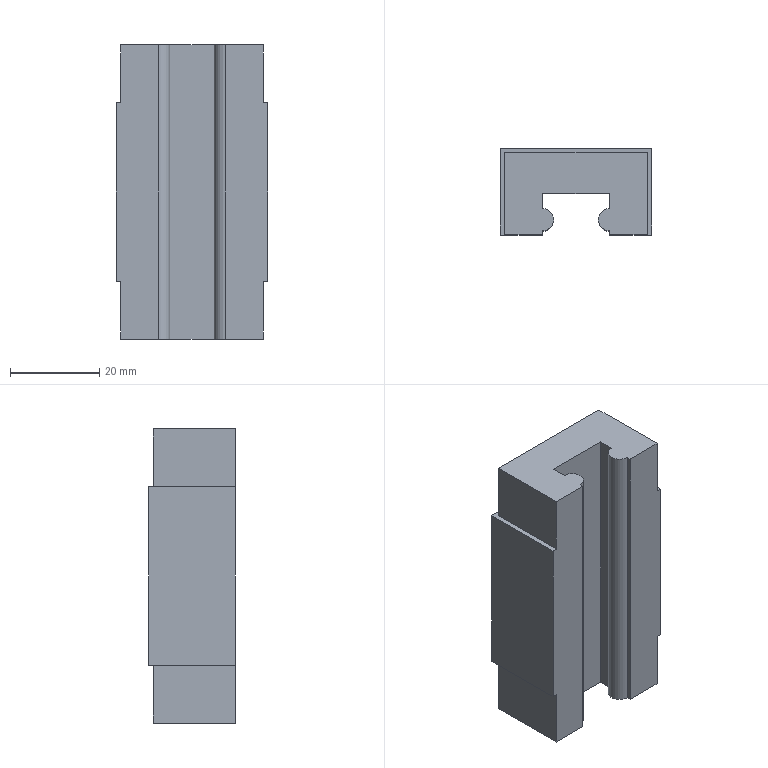Part | Creo | features CURVE 3, DATUM PLANE 3, PROTRUSION 2, COORDINATE SYSTEM 1, CUT 1 | 1 solid | 34 faces | box 34 x 19.41 x 66 mm | volume 33431 mm3 | plane 24 | cylinder 10 | commonest cylinder face diameters 3.3 x8 5 x2
STEP:
#1=CARTESIAN_POINT('',(0.,0.,0.));
#2=DIRECTION('',(0.,0.,1.));
#3=DIRECTION('',(1.,0.,0.));
#4=AXIS2_PLACEMENT_3D('',#1,#2,#3);
#5=CARTESIAN_POINT('',(16.,0.,-20.));
#6=VERTEX_POINT('',#5);
#7=CARTESIAN_POINT('',(16.,18.41,-20.));
#8=VERTEX_POINT('',#7);
#9=CARTESIAN_POINT('',(16.,0.,-20.));
#10=DIRECTION('',(0.,1.,0.));
#11=VECTOR('',#10,18.41);
#12=LINE('',#9,#11);
#13=EDGE_CURVE('',#6,#8,#12,.T.);
#14=ORIENTED_EDGE('',*,*,#13,.F.);
#15=CARTESIAN_POINT('',(17.,0.,-20.));
#16=VERTEX_POINT('',#15);
#17=CARTESIAN_POINT('',(16.,0.,-20.));
#18=DIRECTION('',(1.,0.,0.));
#19=VECTOR('',#18,1.);
#20=LINE('',#17,#19);
#21=EDGE_CURVE('',#6,#16,#20,.T.);
#22=ORIENTED_EDGE('',*,*,#21,.T.);
#23=CARTESIAN_POINT('',(17.,19.41,-20.));
#24=VERTEX_POINT('',#23);
#25=CARTESIAN_POINT('',(17.,0.,-20.));
#26=DIRECTION('',(0.,1.,0.));
#27=VECTOR('',#26,19.41);
#28=LINE('',#25,#27);
#29=EDGE_CURVE('',#16,#24,#28,.T.);
#30=ORIENTED_EDGE('',*,*,#29,.T.);
#31=CARTESIAN_POINT('',(-17.,19.41,-20.));
#32=VERTEX_POINT('',#31);
#33=CARTESIAN_POINT('',(17.,19.41,-20.));
#34=DIRECTION('',(-1.,0.,0.));
#35=VECTOR('',#34,34.);
#36=LINE('',#33,#35);
#37=EDGE_CURVE('',#24,#32,#36,.T.);
#38=ORIENTED_EDGE('',*,*,#37,.T.);
#39=CARTESIAN_POINT('',(-17.,0.,-20.));
#40=VERTEX_POINT('',#39);
#41=CARTESIAN_POINT('',(-17.,19.41,-20.));
#42=DIRECTION('',(0.,-1.,0.));
#43=VECTOR('',#42,19.41);
#44=LINE('',#41,#43);
#45=EDGE_CURVE('',#32,#40,#44,.T.);
#46=ORIENTED_EDGE('',*,*,#45,.T.);
#47=CARTESIAN_POINT('',(-16.,0.,-20.));
#48=VERTEX_POINT('',#47);
#49=CARTESIAN_POINT('',(-17.,0.,-20.));
#50=DIRECTION('',(1.,0.,0.));
#51=VECTOR('',#50,1.);
#52=LINE('',#49,#51);
#53=EDGE_CURVE('',#40,#48,#52,.T.);
#54=ORIENTED_EDGE('',*,*,#53,.T.);
#55=CARTESIAN_POINT('',(-16.,18.41,-20.));
#56=VERTEX_POINT('',#55);
#57=CARTESIAN_POINT('',(-16.,0.,-20.));
#58=DIRECTION('',(0.,1.,0.));
#59=VECTOR('',#58,18.41);
#60=LINE('',#57,#59);
#61=EDGE_CURVE('',#48,#56,#60,.T.);
#62=ORIENTED_EDGE('',*,*,#61,.T.);
#63=CARTESIAN_POINT('',(16.,18.41,-20.));
#64=DIRECTION('',(-1.,0.,0.));
#65=VECTOR('',#64,32.);
#66=LINE('',#63,#65);
#67=EDGE_CURVE('',#8,#56,#66,.T.);
#68=ORIENTED_EDGE('',*,*,#67,.F.);
#69=EDGE_LOOP('',(#14,#22,#30,#38,#46,#54,#62,#68));
#70=FACE_OUTER_BOUND('',#69,.F.);
#71=CARTESIAN_POINT('',(0.,0.,-20.));
#72=DIRECTION('',(0.,0.,1.));
#73=DIRECTION('',(1.,0.,0.));
#74=AXIS2_PLACEMENT_3D('',#71,#72,#73);
#75=PLANE('',#74);
#76=ADVANCED_FACE('',(#70),#75,.F.);
#77=ORIENTED_EDGE('',*,*,#13,.T.);
#78=CARTESIAN_POINT('',(16.,18.41,-33.));
#79=VERTEX_POINT('',#78);
#80=CARTESIAN_POINT('',(16.,18.41,-33.));
#81=DIRECTION('',(0.,0.,1.));
#82=VECTOR('',#81,13.);
#83=LINE('',#80,#82);
#84=EDGE_CURVE('',#79,#8,#83,.T.);
#85=ORIENTED_EDGE('',*,*,#84,.F.);
#86=CARTESIAN_POINT('',(16.,0.,-33.));
#87=VERTEX_POINT('',#86);
#88=CARTESIAN_POINT('',(16.,0.,-33.));
#89=DIRECTION('',(0.,1.,0.));
#90=VECTOR('',#89,18.41);
#91=LINE('',#88,#90);
#92=EDGE_CURVE('',#87,#79,#91,.T.);
#93=ORIENTED_EDGE('',*,*,#92,.F.);
#94=CARTESIAN_POINT('',(16.,0.,-33.));
#95=DIRECTION('',(0.,0.,1.));
#96=VECTOR('',#95,13.);
#97=LINE('',#94,#96);
#98=EDGE_CURVE('',#87,#6,#97,.T.);
#99=ORIENTED_EDGE('',*,*,#98,.T.);
#100=EDGE_LOOP('',(#77,#85,#93,#99));
#101=FACE_OUTER_BOUND('',#100,.F.);
#102=CARTESIAN_POINT('',(16.,0.,-33.));
#103=DIRECTION('',(1.,0.,0.));
#104=DIRECTION('',(0.,1.,0.));
#105=AXIS2_PLACEMENT_3D('',#102,#103,#104);
#106=PLANE('',#105);
#107=ADVANCED_FACE('',(#101),#106,.T.);
#108=CARTESIAN_POINT('',(16.,0.,20.));
#109=VERTEX_POINT('',#108);
#110=CARTESIAN_POINT('',(16.,18.41,20.));
#111=VERTEX_POINT('',#110);
#112=CARTESIAN_POINT('',(16.,0.,20.));
#113=DIRECTION('',(0.,1.,0.));
#114=VECTOR('',#113,18.41);
#115=LINE('',#112,#114);
#116=EDGE_CURVE('',#109,#111,#115,.T.);
#117=ORIENTED_EDGE('',*,*,#116,.F.);
#118=CARTESIAN_POINT('',(16.,0.,33.));
#119=VERTEX_POINT('',#118);
#120=CARTESIAN_POINT('',(16.,0.,20.));
#121=DIRECTION('',(0.,0.,1.));
#122=VECTOR('',#121,13.);
#123=LINE('',#120,#122);
#124=EDGE_CURVE('',#109,#119,#123,.T.);
#125=ORIENTED_EDGE('',*,*,#124,.T.);
#126=CARTESIAN_POINT('',(16.,18.41,33.));
#127=VERTEX_POINT('',#126);
#128=CARTESIAN_POINT('',(16.,0.,33.));
#129=DIRECTION('',(0.,1.,0.));
#130=VECTOR('',#129,18.41);
#131=LINE('',#128,#130);
#132=EDGE_CURVE('',#119,#127,#131,.T.);
#133=ORIENTED_EDGE('',*,*,#132,.T.);
#134=CARTESIAN_POINT('',(16.,18.41,20.));
#135=DIRECTION('',(0.,0.,1.));
#136=VECTOR('',#135,13.);
#137=LINE('',#134,#136);
#138=EDGE_CURVE('',#111,#127,#137,.T.);
#139=ORIENTED_EDGE('',*,*,#138,.F.);
#140=EDGE_LOOP('',(#117,#125,#133,#139));
#141=FACE_OUTER_BOUND('',#140,.F.);
#142=CARTESIAN_POINT('',(16.,0.,-33.));
#143=DIRECTION('',(1.,0.,0.));
#144=DIRECTION('',(0.,1.,0.));
#145=AXIS2_PLACEMENT_3D('',#142,#143,#144);
#146=PLANE('',#145);
#147=ADVANCED_FACE('',(#141),#146,.T.);
#148=ORIENTED_EDGE('',*,*,#67,.T.);
#149=CARTESIAN_POINT('',(-16.,18.41,-33.));
#150=VERTEX_POINT('',#149);
#151=CARTESIAN_POINT('',(-16.,18.41,-33.));
#152=DIRECTION('',(0.,0.,1.));
#153=VECTOR('',#152,13.);
#154=LINE('',#151,#153);
#155=EDGE_CURVE('',#150,#56,#154,.T.);
#156=ORIENTED_EDGE('',*,*,#155,.F.);
#157=CARTESIAN_POINT('',(16.,18.41,-33.));
#158=DIRECTION('',(-1.,0.,0.));
#159=VECTOR('',#158,32.);
#160=LINE('',#157,#159);
#161=EDGE_CURVE('',#79,#150,#160,.T.);
#162=ORIENTED_EDGE('',*,*,#161,.F.);
#163=ORIENTED_EDGE('',*,*,#84,.T.);
#164=EDGE_LOOP('',(#148,#156,#162,#163));
#165=FACE_OUTER_BOUND('',#164,.F.);
#166=CARTESIAN_POINT('',(16.,18.41,-33.));
#167=DIRECTION('',(0.,1.,0.));
#168=DIRECTION('',(-1.,0.,0.));
#169=AXIS2_PLACEMENT_3D('',#166,#167,#168);
#170=PLANE('',#169);
#171=ADVANCED_FACE('',(#165),#170,.T.);
#172=CARTESIAN_POINT('',(-16.,18.41,20.));
#173=VERTEX_POINT('',#172);
#174=CARTESIAN_POINT('',(16.,18.41,20.));
#175=DIRECTION('',(-1.,0.,0.));
#176=VECTOR('',#175,32.);
#177=LINE('',#174,#176);
#178=EDGE_CURVE('',#111,#173,#177,.T.);
#179=ORIENTED_EDGE('',*,*,#178,.F.);
#180=ORIENTED_EDGE('',*,*,#138,.T.);
#181=CARTESIAN_POINT('',(-16.,18.41,33.));
#182=VERTEX_POINT('',#181);
#183=CARTESIAN_POINT('',(16.,18.41,33.));
#184=DIRECTION('',(-1.,0.,0.));
#185=VECTOR('',#184,32.);
#186=LINE('',#183,#185);
#187=EDGE_CURVE('',#127,#182,#186,.T.);
#188=ORIENTED_EDGE('',*,*,#187,.T.);
#189=CARTESIAN_POINT('',(-16.,18.41,20.));
#190=DIRECTION('',(0.,0.,1.));
#191=VECTOR('',#190,13.);
#192=LINE('',#189,#191);
#193=EDGE_CURVE('',#173,#182,#192,.T.);
#194=ORIENTED_EDGE('',*,*,#193,.F.);
#195=EDGE_LOOP('',(#179,#180,#188,#194));
#196=FACE_OUTER_BOUND('',#195,.F.);
#197=CARTESIAN_POINT('',(16.,18.41,-33.));
#198=DIRECTION('',(0.,1.,0.));
#199=DIRECTION('',(-1.,0.,0.));
#200=AXIS2_PLACEMENT_3D('',#197,#198,#199);
#201=PLANE('',#200);
#202=ADVANCED_FACE('',(#196),#201,.T.);
#203=ORIENTED_EDGE('',*,*,#61,.F.);
#204=CARTESIAN_POINT('',(-16.,0.,-33.));
#205=VERTEX_POINT('',#204);
#206=CARTESIAN_POINT('',(-16.,0.,-33.));
#207=DIRECTION('',(0.,0.,1.));
#208=VECTOR('',#207,13.);
#209=LINE('',#206,#208);
#210=EDGE_CURVE('',#205,#48,#209,.T.);
#211=ORIENTED_EDGE('',*,*,#210,.F.);
#212=CARTESIAN_POINT('',(-16.,18.41,-33.));
#213=DIRECTION('',(0.,-1.,0.));
#214=VECTOR('',#213,18.41);
#215=LINE('',#212,#214);
#216=EDGE_CURVE('',#150,#205,#215,.T.);
#217=ORIENTED_EDGE('',*,*,#216,.F.);
#218=ORIENTED_EDGE('',*,*,#155,.T.);
#219=EDGE_LOOP('',(#203,#211,#217,#218));
#220=FACE_OUTER_BOUND('',#219,.F.);
#221=CARTESIAN_POINT('',(-16.,18.41,-33.));
#222=DIRECTION('',(-1.,0.,0.));
#223=DIRECTION('',(0.,-1.,0.));
#224=AXIS2_PLACEMENT_3D('',#221,#222,#223);
#225=PLANE('',#224);
#226=ADVANCED_FACE('',(#220),#225,.T.);
#227=CARTESIAN_POINT('',(-16.,0.,20.));
#228=VERTEX_POINT('',#227);
#229=CARTESIAN_POINT('',(-16.,0.,20.));
#230=DIRECTION('',(0.,1.,0.));
#231=VECTOR('',#230,18.41);
#232=LINE('',#229,#231);
#233=EDGE_CURVE('',#228,#173,#232,.T.);
#234=ORIENTED_EDGE('',*,*,#233,.T.);
#235=ORIENTED_EDGE('',*,*,#193,.T.);
#236=CARTESIAN_POINT('',(-16.,0.,33.));
#237=VERTEX_POINT('',#236);
#238=CARTESIAN_POINT('',(-16.,18.41,33.));
#239=DIRECTION('',(0.,-1.,0.));
#240=VECTOR('',#239,18.41);
#241=LINE('',#238,#240);
#242=EDGE_CURVE('',#182,#237,#241,.T.);
#243=ORIENTED_EDGE('',*,*,#242,.T.);
#244=CARTESIAN_POINT('',(-16.,0.,20.));
#245=DIRECTION('',(0.,0.,1.));
#246=VECTOR('',#245,13.);
#247=LINE('',#244,#246);
#248=EDGE_CURVE('',#228,#237,#247,.T.);
#249=ORIENTED_EDGE('',*,*,#248,.F.);
#250=EDGE_LOOP('',(#234,#235,#243,#249));
#251=FACE_OUTER_BOUND('',#250,.F.);
#252=CARTESIAN_POINT('',(-16.,18.41,-33.));
#253=DIRECTION('',(-1.,0.,0.));
#254=DIRECTION('',(0.,-1.,0.));
#255=AXIS2_PLACEMENT_3D('',#252,#253,#254);
#256=PLANE('',#255);
#257=ADVANCED_FACE('',(#251),#256,.T.);
#258=CARTESIAN_POINT('',(-17.,0.,20.));
#259=VERTEX_POINT('',#258);
#260=CARTESIAN_POINT('',(-17.,0.,20.));
#261=DIRECTION('',(1.,0.,0.));
#262=VECTOR('',#261,1.);
#263=LINE('',#260,#262);
#264=EDGE_CURVE('',#259,#228,#263,.T.);
#265=ORIENTED_EDGE('',*,*,#264,.T.);
#266=ORIENTED_EDGE('',*,*,#248,.T.);
#267=CARTESIAN_POINT('',(-7.5,0.,33.));
#268=VERTEX_POINT('',#267);
#269=CARTESIAN_POINT('',(-16.,0.,33.));
#270=DIRECTION('',(1.,0.,0.));
#271=VECTOR('',#270,8.5);
#272=LINE('',#269,#271);
#273=EDGE_CURVE('',#237,#268,#272,.T.);
#274=ORIENTED_EDGE('',*,*,#273,.T.);
#275=CARTESIAN_POINT('',(-7.5,0.,-33.));
#276=VERTEX_POINT('',#275);
#277=CARTESIAN_POINT('',(-7.5,0.,-33.));
#278=DIRECTION('',(0.,0.,1.));
#279=VECTOR('',#278,66.);
#280=LINE('',#277,#279);
#281=EDGE_CURVE('',#276,#268,#280,.T.);
#282=ORIENTED_EDGE('',*,*,#281,.F.);
#283=CARTESIAN_POINT('',(-16.,0.,-33.));
#284=DIRECTION('',(1.,0.,0.));
#285=VECTOR('',#284,8.5);
#286=LINE('',#283,#285);
#287=EDGE_CURVE('',#205,#276,#286,.T.);
#288=ORIENTED_EDGE('',*,*,#287,.F.);
#289=ORIENTED_EDGE('',*,*,#210,.T.);
#290=ORIENTED_EDGE('',*,*,#53,.F.);
#291=CARTESIAN_POINT('',(-17.,0.,-20.));
#292=DIRECTION('',(0.,0.,1.));
#293=VECTOR('',#292,40.);
#294=LINE('',#291,#293);
#295=EDGE_CURVE('',#40,#259,#294,.T.);
#296=ORIENTED_EDGE('',*,*,#295,.T.);
#297=EDGE_LOOP('',(#265,#266,#274,#282,#288,#289,#290,#296));
#298=FACE_OUTER_BOUND('',#297,.F.);
#299=CARTESIAN_POINT('',(-17.,0.,-20.));
#300=DIRECTION('',(0.,-1.,0.));
#301=DIRECTION('',(1.,0.,0.));
#302=AXIS2_PLACEMENT_3D('',#299,#300,#301);
#303=PLANE('',#302);
#304=ADVANCED_FACE('',(#298),#303,.T.);
#305=ORIENTED_EDGE('',*,*,#116,.T.);
#306=ORIENTED_EDGE('',*,*,#178,.T.);
#307=ORIENTED_EDGE('',*,*,#233,.F.);
#308=ORIENTED_EDGE('',*,*,#264,.F.);
#309=CARTESIAN_POINT('',(-17.,19.41,20.));
#310=VERTEX_POINT('',#309);
#311=CARTESIAN_POINT('',(-17.,19.41,20.));
#312=DIRECTION('',(0.,-1.,0.));
#313=VECTOR('',#312,19.41);
#314=LINE('',#311,#313);
#315=EDGE_CURVE('',#310,#259,#314,.T.);
#316=ORIENTED_EDGE('',*,*,#315,.F.);
#317=CARTESIAN_POINT('',(17.,19.41,20.));
#318=VERTEX_POINT('',#317);
#319=CARTESIAN_POINT('',(17.,19.41,20.));
#320=DIRECTION('',(-1.,0.,0.));
#321=VECTOR('',#320,34.);
#322=LINE('',#319,#321);
#323=EDGE_CURVE('',#318,#310,#322,.T.);
#324=ORIENTED_EDGE('',*,*,#323,.F.);
#325=CARTESIAN_POINT('',(17.,0.,20.));
#326=VERTEX_POINT('',#325);
#327=CARTESIAN_POINT('',(17.,0.,20.));
#328=DIRECTION('',(0.,1.,0.));
#329=VECTOR('',#328,19.41);
#330=LINE('',#327,#329);
#331=EDGE_CURVE('',#326,#318,#330,.T.);
#332=ORIENTED_EDGE('',*,*,#331,.F.);
#333=CARTESIAN_POINT('',(16.,0.,20.));
#334=DIRECTION('',(1.,0.,0.));
#335=VECTOR('',#334,1.);
#336=LINE('',#333,#335);
#337=EDGE_CURVE('',#109,#326,#336,.T.);
#338=ORIENTED_EDGE('',*,*,#337,.F.);
#339=EDGE_LOOP('',(#305,#306,#307,#308,#316,#324,#332,#338));
#340=FACE_OUTER_BOUND('',#339,.F.);
#341=CARTESIAN_POINT('',(0.,0.,20.));
#342=DIRECTION('',(0.,0.,1.));
#343=DIRECTION('',(1.,0.,0.));
#344=AXIS2_PLACEMENT_3D('',#341,#342,#343);
#345=PLANE('',#344);
#346=ADVANCED_FACE('',(#340),#345,.T.);
#347=ORIENTED_EDGE('',*,*,#45,.F.);
#348=CARTESIAN_POINT('',(-17.,19.41,-20.));
#349=DIRECTION('',(0.,0.,1.));
#350=VECTOR('',#349,40.);
#351=LINE('',#348,#350);
#352=EDGE_CURVE('',#32,#310,#351,.T.);
#353=ORIENTED_EDGE('',*,*,#352,.T.);
#354=ORIENTED_EDGE('',*,*,#315,.T.);
#355=ORIENTED_EDGE('',*,*,#295,.F.);
#356=EDGE_LOOP('',(#347,#353,#354,#355));
#357=FACE_OUTER_BOUND('',#356,.F.);
#358=CARTESIAN_POINT('',(-17.,19.41,-20.));
#359=DIRECTION('',(-1.,0.,0.));
#360=DIRECTION('',(0.,-1.,0.));
#361=AXIS2_PLACEMENT_3D('',#358,#359,#360);
#362=PLANE('',#361);
#363=ADVANCED_FACE('',(#357),#362,.T.);
#364=ORIENTED_EDGE('',*,*,#37,.F.);
#365=CARTESIAN_POINT('',(17.,19.41,-20.));
#366=DIRECTION('',(0.,0.,1.));
#367=VECTOR('',#366,40.);
#368=LINE('',#365,#367);
#369=EDGE_CURVE('',#24,#318,#368,.T.);
#370=ORIENTED_EDGE('',*,*,#369,.T.);
#371=ORIENTED_EDGE('',*,*,#323,.T.);
#372=ORIENTED_EDGE('',*,*,#352,.F.);
#373=EDGE_LOOP('',(#364,#370,#371,#372));
#374=FACE_OUTER_BOUND('',#373,.F.);
#375=CARTESIAN_POINT('',(14.65,19.41,-13.));
#376=VERTEX_POINT('',#375);
#377=CARTESIAN_POINT('',(11.35,19.41,-13.));
#378=VERTEX_POINT('',#377);
#379=CARTESIAN_POINT('',(13.,19.41,-13.));
#380=DIRECTION('',(0.,1.,0.));
#381=DIRECTION('',(1.,0.,0.));
#382=AXIS2_PLACEMENT_3D('',#379,#380,#381);
#383=CIRCLE('',#382,1.65);
#384=EDGE_CURVE('',#376,#378,#383,.T.);
#385=ORIENTED_EDGE('',*,*,#384,.T.);
#386=CARTESIAN_POINT('',(13.,19.41,-13.));
#387=DIRECTION('',(0.,1.,0.));
#388=DIRECTION('',(-1.,0.,0.));
#389=AXIS2_PLACEMENT_3D('',#386,#387,#388);
#390=CIRCLE('',#389,1.65);
#391=EDGE_CURVE('',#378,#376,#390,.T.);
#392=ORIENTED_EDGE('',*,*,#391,.T.);
#393=EDGE_LOOP('',(#385,#392));
#394=FACE_BOUND('',#393,.F.);
#395=CARTESIAN_POINT('',(-11.35,19.41,-13.));
#396=VERTEX_POINT('',#395);
#397=CARTESIAN_POINT('',(-14.65,19.41,-13.));
#398=VERTEX_POINT('',#397);
#399=CARTESIAN_POINT('',(-13.,19.41,-13.));
#400=DIRECTION('',(0.,1.,0.));
#401=DIRECTION('',(1.,0.,0.));
#402=AXIS2_PLACEMENT_3D('',#399,#400,#401);
#403=CIRCLE('',#402,1.65);
#404=EDGE_CURVE('',#396,#398,#403,.T.);
#405=ORIENTED_EDGE('',*,*,#404,.T.);
#406=CARTESIAN_POINT('',(-13.,19.41,-13.));
#407=DIRECTION('',(0.,1.,0.));
#408=DIRECTION('',(-1.,0.,0.));
#409=AXIS2_PLACEMENT_3D('',#406,#407,#408);
#410=CIRCLE('',#409,1.65);
#411=EDGE_CURVE('',#398,#396,#410,.T.);
#412=ORIENTED_EDGE('',*,*,#411,.T.);
#413=EDGE_LOOP('',(#405,#412));
#414=FACE_BOUND('',#413,.F.);
#415=CARTESIAN_POINT('',(-11.35,19.41,13.));
#416=VERTEX_POINT('',#415);
#417=CARTESIAN_POINT('',(-14.65,19.41,13.));
#418=VERTEX_POINT('',#417);
#419=CARTESIAN_POINT('',(-13.,19.41,13.));
#420=DIRECTION('',(0.,1.,0.));
#421=DIRECTION('',(1.,0.,0.));
#422=AXIS2_PLACEMENT_3D('',#419,#420,#421);
#423=CIRCLE('',#422,1.65);
#424=EDGE_CURVE('',#416,#418,#423,.T.);
#425=ORIENTED_EDGE('',*,*,#424,.T.);
#426=CARTESIAN_POINT('',(-13.,19.41,13.));
#427=DIRECTION('',(0.,1.,0.));
#428=DIRECTION('',(-1.,0.,0.));
#429=AXIS2_PLACEMENT_3D('',#426,#427,#428);
#430=CIRCLE('',#429,1.65);
#431=EDGE_CURVE('',#418,#416,#430,.T.);
#432=ORIENTED_EDGE('',*,*,#431,.T.);
#433=EDGE_LOOP('',(#425,#432));
#434=FACE_BOUND('',#433,.F.);
#435=CARTESIAN_POINT('',(14.65,19.41,13.));
#436=VERTEX_POINT('',#435);
#437=CARTESIAN_POINT('',(11.35,19.41,13.));
#438=VERTEX_POINT('',#437);
#439=CARTESIAN_POINT('',(13.,19.41,13.));
#440=DIRECTION('',(0.,1.,0.));
#441=DIRECTION('',(1.,0.,0.));
#442=AXIS2_PLACEMENT_3D('',#439,#440,#441);
#443=CIRCLE('',#442,1.65);
#444=EDGE_CURVE('',#436,#438,#443,.T.);
#445=ORIENTED_EDGE('',*,*,#444,.T.);
#446=CARTESIAN_POINT('',(13.,19.41,13.));
#447=DIRECTION('',(0.,1.,0.));
#448=DIRECTION('',(-1.,0.,0.));
#449=AXIS2_PLACEMENT_3D('',#446,#447,#448);
#450=CIRCLE('',#449,1.65);
#451=EDGE_CURVE('',#438,#436,#450,.T.);
#452=ORIENTED_EDGE('',*,*,#451,.T.);
#453=EDGE_LOOP('',(#445,#452));
#454=FACE_BOUND('',#453,.F.);
#455=CARTESIAN_POINT('',(17.,19.41,-20.));
#456=DIRECTION('',(0.,1.,0.));
#457=DIRECTION('',(-1.,0.,0.));
#458=AXIS2_PLACEMENT_3D('',#455,#456,#457);
#459=PLANE('',#458);
#460=ADVANCED_FACE('',(#374,#394,#414,#434,#454),#459,.T.);
#461=ORIENTED_EDGE('',*,*,#29,.F.);
#462=CARTESIAN_POINT('',(17.,0.,-20.));
#463=DIRECTION('',(0.,0.,1.));
#464=VECTOR('',#463,40.);
#465=LINE('',#462,#464);
#466=EDGE_CURVE('',#16,#326,#465,.T.);
#467=ORIENTED_EDGE('',*,*,#466,.T.);
#468=ORIENTED_EDGE('',*,*,#331,.T.);
#469=ORIENTED_EDGE('',*,*,#369,.F.);
#470=EDGE_LOOP('',(#461,#467,#468,#469));
#471=FACE_OUTER_BOUND('',#470,.F.);
#472=CARTESIAN_POINT('',(17.,0.,-20.));
#473=DIRECTION('',(1.,0.,0.));
#474=DIRECTION('',(0.,1.,0.));
#475=AXIS2_PLACEMENT_3D('',#472,#473,#474);
#476=PLANE('',#475);
#477=ADVANCED_FACE('',(#471),#476,.T.);
#478=CARTESIAN_POINT('',(7.5,0.,-33.));
#479=VERTEX_POINT('',#478);
#480=CARTESIAN_POINT('',(7.5,0.,33.));
#481=VERTEX_POINT('',#480);
#482=CARTESIAN_POINT('',(7.5,0.,-33.));
#483=DIRECTION('',(0.,0.,1.));
#484=VECTOR('',#483,66.);
#485=LINE('',#482,#484);
#486=EDGE_CURVE('',#479,#481,#485,.T.);
#487=ORIENTED_EDGE('',*,*,#486,.T.);
#488=CARTESIAN_POINT('',(7.5,0.,33.));
#489=DIRECTION('',(1.,0.,0.));
#490=VECTOR('',#489,8.5);
#491=LINE('',#488,#490);
#492=EDGE_CURVE('',#481,#119,#491,.T.);
#493=ORIENTED_EDGE('',*,*,#492,.T.);
#494=ORIENTED_EDGE('',*,*,#124,.F.);
#495=ORIENTED_EDGE('',*,*,#337,.T.);
#496=ORIENTED_EDGE('',*,*,#466,.F.);
#497=ORIENTED_EDGE('',*,*,#21,.F.);
#498=ORIENTED_EDGE('',*,*,#98,.F.);
#499=CARTESIAN_POINT('',(7.5,0.,-33.));
#500=DIRECTION('',(1.,0.,0.));
#501=VECTOR('',#500,8.5);
#502=LINE('',#499,#501);
#503=EDGE_CURVE('',#479,#87,#502,.T.);
#504=ORIENTED_EDGE('',*,*,#503,.F.);
#505=EDGE_LOOP('',(#487,#493,#494,#495,#496,#497,#498,#504));
#506=FACE_OUTER_BOUND('',#505,.F.);
#507=CARTESIAN_POINT('',(7.5,0.,-20.));
#508=DIRECTION('',(0.,-1.,0.));
#509=DIRECTION('',(1.,0.,0.));
#510=AXIS2_PLACEMENT_3D('',#507,#508,#509);
#511=PLANE('',#510);
#512=ADVANCED_FACE('',(#506),#511,.T.);
#513=CARTESIAN_POINT('',(7.5,0.9,-33.));
#514=VERTEX_POINT('',#513);
#515=CARTESIAN_POINT('',(7.5,0.9,33.));
#516=VERTEX_POINT('',#515);
#517=CARTESIAN_POINT('',(7.5,0.9,-33.));
#518=DIRECTION('',(0.,0.,1.));
#519=VECTOR('',#518,66.);
#520=LINE('',#517,#519);
#521=EDGE_CURVE('',#514,#516,#520,.T.);
#522=ORIENTED_EDGE('',*,*,#521,.T.);
#523=CARTESIAN_POINT('',(7.5,0.9,33.));
#524=DIRECTION('',(0.,-1.,0.));
#525=VECTOR('',#524,0.9);
#526=LINE('',#523,#525);
#527=EDGE_CURVE('',#516,#481,#526,.T.);
#528=ORIENTED_EDGE('',*,*,#527,.T.);
#529=ORIENTED_EDGE('',*,*,#486,.F.);
#530=CARTESIAN_POINT('',(7.5,0.9,-33.));
#531=DIRECTION('',(0.,-1.,0.));
#532=VECTOR('',#531,0.9);
#533=LINE('',#530,#532);
#534=EDGE_CURVE('',#514,#479,#533,.T.);
#535=ORIENTED_EDGE('',*,*,#534,.F.);
#536=EDGE_LOOP('',(#522,#528,#529,#535));
#537=FACE_OUTER_BOUND('',#536,.F.);
#538=CARTESIAN_POINT('',(7.5,0.9,-20.));
#539=DIRECTION('',(-1.,0.,0.));
#540=DIRECTION('',(0.,-1.,0.));
#541=AXIS2_PLACEMENT_3D('',#538,#539,#540);
#542=PLANE('',#541);
#543=ADVANCED_FACE('',(#537),#542,.T.);
#544=CARTESIAN_POINT('',(7.5,5.9,-33.));
#545=VERTEX_POINT('',#544);
#546=CARTESIAN_POINT('',(7.5,5.9,33.));
#547=VERTEX_POINT('',#546);
#548=CARTESIAN_POINT('',(7.5,5.9,-33.));
#549=DIRECTION('',(0.,0.,1.));
#550=VECTOR('',#549,66.);
#551=LINE('',#548,#550);
#552=EDGE_CURVE('',#545,#547,#551,.T.);
#553=ORIENTED_EDGE('',*,*,#552,.T.);
#554=CARTESIAN_POINT('',(7.5,3.4,33.));
#555=DIRECTION('',(0.,0.,1.));
#556=DIRECTION('',(0.,1.,0.));
#557=AXIS2_PLACEMENT_3D('',#554,#555,#556);
#558=CIRCLE('',#557,2.5);
#559=EDGE_CURVE('',#547,#516,#558,.T.);
#560=ORIENTED_EDGE('',*,*,#559,.T.);
#561=ORIENTED_EDGE('',*,*,#521,.F.);
#562=CARTESIAN_POINT('',(7.5,3.4,-33.));
#563=DIRECTION('',(0.,0.,1.));
#564=DIRECTION('',(0.,1.,0.));
#565=AXIS2_PLACEMENT_3D('',#562,#563,#564);
#566=CIRCLE('',#565,2.5);
#567=EDGE_CURVE('',#545,#514,#566,.T.);
#568=ORIENTED_EDGE('',*,*,#567,.F.);
#569=EDGE_LOOP('',(#553,#560,#561,#568));
#570=FACE_OUTER_BOUND('',#569,.F.);
#571=CARTESIAN_POINT('',(7.5,3.4,-20.));
#572=DIRECTION('',(0.,0.,1.));
#573=DIRECTION('',(1.,0.,0.));
#574=AXIS2_PLACEMENT_3D('',#571,#572,#573);
#575=CYLINDRICAL_SURFACE('',#574,2.5);
#576=ADVANCED_FACE('',(#570),#575,.T.);
#577=CARTESIAN_POINT('',(7.5,9.4,-33.));
#578=VERTEX_POINT('',#577);
#579=CARTESIAN_POINT('',(7.5,9.4,33.));
#580=VERTEX_POINT('',#579);
#581=CARTESIAN_POINT('',(7.5,9.4,-33.));
#582=DIRECTION('',(0.,0.,1.));
#583=VECTOR('',#582,66.);
#584=LINE('',#581,#583);
#585=EDGE_CURVE('',#578,#580,#584,.T.);
#586=ORIENTED_EDGE('',*,*,#585,.T.);
#587=CARTESIAN_POINT('',(7.5,9.4,33.));
#588=DIRECTION('',(0.,-1.,0.));
#589=VECTOR('',#588,3.5);
#590=LINE('',#587,#589);
#591=EDGE_CURVE('',#580,#547,#590,.T.);
#592=ORIENTED_EDGE('',*,*,#591,.T.);
#593=ORIENTED_EDGE('',*,*,#552,.F.);
#594=CARTESIAN_POINT('',(7.5,9.4,-33.));
#595=DIRECTION('',(0.,-1.,0.));
#596=VECTOR('',#595,3.5);
#597=LINE('',#594,#596);
#598=EDGE_CURVE('',#578,#545,#597,.T.);
#599=ORIENTED_EDGE('',*,*,#598,.F.);
#600=EDGE_LOOP('',(#586,#592,#593,#599));
#601=FACE_OUTER_BOUND('',#600,.F.);
#602=CARTESIAN_POINT('',(7.5,9.4,-20.));
#603=DIRECTION('',(-1.,0.,0.));
#604=DIRECTION('',(0.,-1.,0.));
#605=AXIS2_PLACEMENT_3D('',#602,#603,#604);
#606=PLANE('',#605);
#607=ADVANCED_FACE('',(#601),#606,.T.);
#608=CARTESIAN_POINT('',(-7.5,9.4,-33.));
#609=VERTEX_POINT('',#608);
#610=CARTESIAN_POINT('',(-7.5,9.4,33.));
#611=VERTEX_POINT('',#610);
#612=CARTESIAN_POINT('',(-7.5,9.4,-33.));
#613=DIRECTION('',(0.,0.,1.));
#614=VECTOR('',#613,66.);
#615=LINE('',#612,#614);
#616=EDGE_CURVE('',#609,#611,#615,.T.);
#617=ORIENTED_EDGE('',*,*,#616,.T.);
#618=CARTESIAN_POINT('',(-7.5,9.4,33.));
#619=DIRECTION('',(1.,0.,0.));
#620=VECTOR('',#619,15.);
#621=LINE('',#618,#620);
#622=EDGE_CURVE('',#611,#580,#621,.T.);
#623=ORIENTED_EDGE('',*,*,#622,.T.);
#624=ORIENTED_EDGE('',*,*,#585,.F.);
#625=CARTESIAN_POINT('',(-7.5,9.4,-33.));
#626=DIRECTION('',(1.,0.,0.));
#627=VECTOR('',#626,15.);
#628=LINE('',#625,#627);
#629=EDGE_CURVE('',#609,#578,#628,.T.);
#630=ORIENTED_EDGE('',*,*,#629,.F.);
#631=EDGE_LOOP('',(#617,#623,#624,#630));
#632=FACE_OUTER_BOUND('',#631,.F.);
#633=CARTESIAN_POINT('',(-7.5,9.4,-20.));
#634=DIRECTION('',(0.,-1.,0.));
#635=DIRECTION('',(1.,0.,0.));
#636=AXIS2_PLACEMENT_3D('',#633,#634,#635);
#637=PLANE('',#636);
#638=ADVANCED_FACE('',(#632),#637,.T.);
#639=CARTESIAN_POINT('',(-7.5,5.9,-33.));
#640=VERTEX_POINT('',#639);
#641=CARTESIAN_POINT('',(-7.5,5.9,33.));
#642=VERTEX_POINT('',#641);
#643=CARTESIAN_POINT('',(-7.5,5.9,-33.));
#644=DIRECTION('',(0.,0.,1.));
#645=VECTOR('',#644,66.);
#646=LINE('',#643,#645);
#647=EDGE_CURVE('',#640,#642,#646,.T.);
#648=ORIENTED_EDGE('',*,*,#647,.T.);
#649=CARTESIAN_POINT('',(-7.5,5.9,33.));
#650=DIRECTION('',(0.,1.,0.));
#651=VECTOR('',#650,3.5);
#652=LINE('',#649,#651);
#653=EDGE_CURVE('',#642,#611,#652,.T.);
#654=ORIENTED_EDGE('',*,*,#653,.T.);
#655=ORIENTED_EDGE('',*,*,#616,.F.);
#656=CARTESIAN_POINT('',(-7.5,5.9,-33.));
#657=DIRECTION('',(0.,1.,0.));
#658=VECTOR('',#657,3.5);
#659=LINE('',#656,#658);
#660=EDGE_CURVE('',#640,#609,#659,.T.);
#661=ORIENTED_EDGE('',*,*,#660,.F.);
#662=EDGE_LOOP('',(#648,#654,#655,#661));
#663=FACE_OUTER_BOUND('',#662,.F.);
#664=CARTESIAN_POINT('',(-7.5,5.9,-20.));
#665=DIRECTION('',(1.,0.,0.));
#666=DIRECTION('',(0.,1.,0.));
#667=AXIS2_PLACEMENT_3D('',#664,#665,#666);
#668=PLANE('',#667);
#669=ADVANCED_FACE('',(#663),#668,.T.);
#670=CARTESIAN_POINT('',(-7.5,0.9,-33.));
#671=VERTEX_POINT('',#670);
#672=CARTESIAN_POINT('',(-7.5,0.9,33.));
#673=VERTEX_POINT('',#672);
#674=CARTESIAN_POINT('',(-7.5,0.9,-33.));
#675=DIRECTION('',(0.,0.,1.));
#676=VECTOR('',#675,66.);
#677=LINE('',#674,#676);
#678=EDGE_CURVE('',#671,#673,#677,.T.);
#679=ORIENTED_EDGE('',*,*,#678,.T.);
#680=CARTESIAN_POINT('',(-7.5,3.4,33.));
#681=DIRECTION('',(0.,0.,1.));
#682=DIRECTION('',(0.,-1.,0.));
#683=AXIS2_PLACEMENT_3D('',#680,#681,#682);
#684=CIRCLE('',#683,2.5);
#685=EDGE_CURVE('',#673,#642,#684,.T.);
#686=ORIENTED_EDGE('',*,*,#685,.T.);
#687=ORIENTED_EDGE('',*,*,#647,.F.);
#688=CARTESIAN_POINT('',(-7.5,3.4,-33.));
#689=DIRECTION('',(0.,0.,1.));
#690=DIRECTION('',(0.,-1.,0.));
#691=AXIS2_PLACEMENT_3D('',#688,#689,#690);
#692=CIRCLE('',#691,2.5);
#693=EDGE_CURVE('',#671,#640,#692,.T.);
#694=ORIENTED_EDGE('',*,*,#693,.F.);
#695=EDGE_LOOP('',(#679,#686,#687,#694));
#696=FACE_OUTER_BOUND('',#695,.F.);
#697=CARTESIAN_POINT('',(-7.5,3.4,-20.));
#698=DIRECTION('',(0.,0.,1.));
#699=DIRECTION('',(1.,0.,0.));
#700=AXIS2_PLACEMENT_3D('',#697,#698,#699);
#701=CYLINDRICAL_SURFACE('',#700,2.5);
#702=ADVANCED_FACE('',(#696),#701,.T.);
#703=ORIENTED_EDGE('',*,*,#281,.T.);
#704=CARTESIAN_POINT('',(-7.5,0.,33.));
#705=DIRECTION('',(0.,1.,0.));
#706=VECTOR('',#705,0.9);
#707=LINE('',#704,#706);
#708=EDGE_CURVE('',#268,#673,#707,.T.);
#709=ORIENTED_EDGE('',*,*,#708,.T.);
#710=ORIENTED_EDGE('',*,*,#678,.F.);
#711=CARTESIAN_POINT('',(-7.5,0.,-33.));
#712=DIRECTION('',(0.,1.,0.));
#713=VECTOR('',#712,0.9);
#714=LINE('',#711,#713);
#715=EDGE_CURVE('',#276,#671,#714,.T.);
#716=ORIENTED_EDGE('',*,*,#715,.F.);
#717=EDGE_LOOP('',(#703,#709,#710,#716));
#718=FACE_OUTER_BOUND('',#717,.F.);
#719=CARTESIAN_POINT('',(-7.5,0.,-20.));
#720=DIRECTION('',(1.,0.,0.));
#721=DIRECTION('',(0.,1.,0.));
#722=AXIS2_PLACEMENT_3D('',#719,#720,#721);
#723=PLANE('',#722);
#724=ADVANCED_FACE('',(#718),#723,.T.);
#725=ORIENTED_EDGE('',*,*,#132,.F.);
#726=ORIENTED_EDGE('',*,*,#492,.F.);
#727=ORIENTED_EDGE('',*,*,#527,.F.);
#728=ORIENTED_EDGE('',*,*,#559,.F.);
#729=ORIENTED_EDGE('',*,*,#591,.F.);
#730=ORIENTED_EDGE('',*,*,#622,.F.);
#731=ORIENTED_EDGE('',*,*,#653,.F.);
#732=ORIENTED_EDGE('',*,*,#685,.F.);
#733=ORIENTED_EDGE('',*,*,#708,.F.);
#734=ORIENTED_EDGE('',*,*,#273,.F.);
#735=ORIENTED_EDGE('',*,*,#242,.F.);
#736=ORIENTED_EDGE('',*,*,#187,.F.);
#737=EDGE_LOOP('',(#725,#726,#727,#728,#729,#730,#731,#732,#733,#734,#735,#736));
#738=FACE_OUTER_BOUND('',#737,.F.);
#739=CARTESIAN_POINT('',(0.,0.,33.));
#740=DIRECTION('',(0.,0.,1.));
#741=DIRECTION('',(1.,0.,0.));
#742=AXIS2_PLACEMENT_3D('',#739,#740,#741);
#743=PLANE('',#742);
#744=ADVANCED_FACE('',(#738),#743,.T.);
#745=ORIENTED_EDGE('',*,*,#92,.T.);
#746=ORIENTED_EDGE('',*,*,#161,.T.);
#747=ORIENTED_EDGE('',*,*,#216,.T.);
#748=ORIENTED_EDGE('',*,*,#287,.T.);
#749=ORIENTED_EDGE('',*,*,#715,.T.);
#750=ORIENTED_EDGE('',*,*,#693,.T.);
#751=ORIENTED_EDGE('',*,*,#660,.T.);
#752=ORIENTED_EDGE('',*,*,#629,.T.);
#753=ORIENTED_EDGE('',*,*,#598,.T.);
#754=ORIENTED_EDGE('',*,*,#567,.T.);
#755=ORIENTED_EDGE('',*,*,#534,.T.);
#756=ORIENTED_EDGE('',*,*,#503,.T.);
#757=EDGE_LOOP('',(#745,#746,#747,#748,#749,#750,#751,#752,#753,#754,#755,#756));
#758=FACE_OUTER_BOUND('',#757,.F.);
#759=CARTESIAN_POINT('',(0.,0.,-33.));
#760=DIRECTION('',(0.,0.,1.));
#761=DIRECTION('',(1.,0.,0.));
#762=AXIS2_PLACEMENT_3D('',#759,#760,#761);
#763=PLANE('',#762);
#764=ADVANCED_FACE('',(#758),#763,.F.);
#765=ORIENTED_EDGE('',*,*,#384,.F.);
#766=CARTESIAN_POINT('',(14.65,11.41,-13.));
#767=VERTEX_POINT('',#766);
#768=CARTESIAN_POINT('',(14.65,19.41,-13.));
#769=DIRECTION('',(0.,-1.,0.));
#770=VECTOR('',#769,8.);
#771=LINE('',#768,#770);
#772=EDGE_CURVE('',#376,#767,#771,.T.);
#773=ORIENTED_EDGE('',*,*,#772,.T.);
#774=CARTESIAN_POINT('',(11.35,11.41,-13.));
#775=VERTEX_POINT('',#774);
#776=CARTESIAN_POINT('',(13.,11.41,-13.));
#777=DIRECTION('',(0.,1.,0.));
#778=DIRECTION('',(1.,0.,0.));
#779=AXIS2_PLACEMENT_3D('',#776,#777,#778);
#780=CIRCLE('',#779,1.65);
#781=EDGE_CURVE('',#767,#775,#780,.T.);
#782=ORIENTED_EDGE('',*,*,#781,.T.);
#783=CARTESIAN_POINT('',(11.35,19.41,-13.));
#784=DIRECTION('',(0.,-1.,0.));
#785=VECTOR('',#784,8.);
#786=LINE('',#783,#785);
#787=EDGE_CURVE('',#378,#775,#786,.T.);
#788=ORIENTED_EDGE('',*,*,#787,.F.);
#789=EDGE_LOOP('',(#765,#773,#782,#788));
#790=FACE_OUTER_BOUND('',#789,.F.);
#791=CARTESIAN_POINT('',(13.,19.41,-13.));
#792=DIRECTION('',(0.,1.,0.));
#793=DIRECTION('',(1.,0.,0.));
#794=AXIS2_PLACEMENT_3D('',#791,#792,#793);
#795=CYLINDRICAL_SURFACE('',#794,1.65);
#796=ADVANCED_FACE('',(#790),#795,.F.);
#797=ORIENTED_EDGE('',*,*,#391,.F.);
#798=ORIENTED_EDGE('',*,*,#787,.T.);
#799=CARTESIAN_POINT('',(13.,11.41,-13.));
#800=DIRECTION('',(0.,1.,0.));
#801=DIRECTION('',(-1.,0.,0.));
#802=AXIS2_PLACEMENT_3D('',#799,#800,#801);
#803=CIRCLE('',#802,1.65);
#804=EDGE_CURVE('',#775,#767,#803,.T.);
#805=ORIENTED_EDGE('',*,*,#804,.T.);
#806=ORIENTED_EDGE('',*,*,#772,.F.);
#807=EDGE_LOOP('',(#797,#798,#805,#806));
#808=FACE_OUTER_BOUND('',#807,.F.);
#809=CARTESIAN_POINT('',(13.,19.41,-13.));
#810=DIRECTION('',(0.,1.,0.));
#811=DIRECTION('',(1.,0.,0.));
#812=AXIS2_PLACEMENT_3D('',#809,#810,#811);
#813=CYLINDRICAL_SURFACE('',#812,1.65);
#814=ADVANCED_FACE('',(#808),#813,.F.);
#815=ORIENTED_EDGE('',*,*,#781,.F.);
#816=ORIENTED_EDGE('',*,*,#804,.F.);
#817=EDGE_LOOP('',(#815,#816));
#818=FACE_OUTER_BOUND('',#817,.F.);
#819=CARTESIAN_POINT('',(0.,11.41,-20.));
#820=DIRECTION('',(0.,1.,0.));
#821=DIRECTION('',(1.,0.,0.));
#822=AXIS2_PLACEMENT_3D('',#819,#820,#821);
#823=PLANE('',#822);
#824=ADVANCED_FACE('',(#818),#823,.T.);
#825=CARTESIAN_POINT('',(-11.35,11.41,-13.));
#826=VERTEX_POINT('',#825);
#827=CARTESIAN_POINT('',(-14.65,11.41,-13.));
#828=VERTEX_POINT('',#827);
#829=CARTESIAN_POINT('',(-13.,11.41,-13.));
#830=DIRECTION('',(0.,1.,0.));
#831=DIRECTION('',(1.,0.,0.));
#832=AXIS2_PLACEMENT_3D('',#829,#830,#831);
#833=CIRCLE('',#832,1.65);
#834=EDGE_CURVE('',#826,#828,#833,.T.);
#835=ORIENTED_EDGE('',*,*,#834,.F.);
#836=CARTESIAN_POINT('',(-13.,11.41,-13.));
#837=DIRECTION('',(0.,1.,0.));
#838=DIRECTION('',(-1.,0.,0.));
#839=AXIS2_PLACEMENT_3D('',#836,#837,#838);
#840=CIRCLE('',#839,1.65);
#841=EDGE_CURVE('',#828,#826,#840,.T.);
#842=ORIENTED_EDGE('',*,*,#841,.F.);
#843=EDGE_LOOP('',(#835,#842));
#844=FACE_OUTER_BOUND('',#843,.F.);
#845=CARTESIAN_POINT('',(0.,11.41,-20.));
#846=DIRECTION('',(0.,1.,0.));
#847=DIRECTION('',(1.,0.,0.));
#848=AXIS2_PLACEMENT_3D('',#845,#846,#847);
#849=PLANE('',#848);
#850=ADVANCED_FACE('',(#844),#849,.T.);
#851=CARTESIAN_POINT('',(-11.35,11.41,13.));
#852=VERTEX_POINT('',#851);
#853=CARTESIAN_POINT('',(-14.65,11.41,13.));
#854=VERTEX_POINT('',#853);
#855=CARTESIAN_POINT('',(-13.,11.41,13.));
#856=DIRECTION('',(0.,1.,0.));
#857=DIRECTION('',(1.,0.,0.));
#858=AXIS2_PLACEMENT_3D('',#855,#856,#857);
#859=CIRCLE('',#858,1.65);
#860=EDGE_CURVE('',#852,#854,#859,.T.);
#861=ORIENTED_EDGE('',*,*,#860,.F.);
#862=CARTESIAN_POINT('',(-13.,11.41,13.));
#863=DIRECTION('',(0.,1.,0.));
#864=DIRECTION('',(-1.,0.,0.));
#865=AXIS2_PLACEMENT_3D('',#862,#863,#864);
#866=CIRCLE('',#865,1.65);
#867=EDGE_CURVE('',#854,#852,#866,.T.);
#868=ORIENTED_EDGE('',*,*,#867,.F.);
#869=EDGE_LOOP('',(#861,#868));
#870=FACE_OUTER_BOUND('',#869,.F.);
#871=CARTESIAN_POINT('',(0.,11.41,-20.));
#872=DIRECTION('',(0.,1.,0.));
#873=DIRECTION('',(1.,0.,0.));
#874=AXIS2_PLACEMENT_3D('',#871,#872,#873);
#875=PLANE('',#874);
#876=ADVANCED_FACE('',(#870),#875,.T.);
#877=CARTESIAN_POINT('',(14.65,11.41,13.));
#878=VERTEX_POINT('',#877);
#879=CARTESIAN_POINT('',(11.35,11.41,13.));
#880=VERTEX_POINT('',#879);
#881=CARTESIAN_POINT('',(13.,11.41,13.));
#882=DIRECTION('',(0.,1.,0.));
#883=DIRECTION('',(1.,0.,0.));
#884=AXIS2_PLACEMENT_3D('',#881,#882,#883);
#885=CIRCLE('',#884,1.65);
#886=EDGE_CURVE('',#878,#880,#885,.T.);
#887=ORIENTED_EDGE('',*,*,#886,.F.);
#888=CARTESIAN_POINT('',(13.,11.41,13.));
#889=DIRECTION('',(0.,1.,0.));
#890=DIRECTION('',(-1.,0.,0.));
#891=AXIS2_PLACEMENT_3D('',#888,#889,#890);
#892=CIRCLE('',#891,1.65);
#893=EDGE_CURVE('',#880,#878,#892,.T.);
#894=ORIENTED_EDGE('',*,*,#893,.F.);
#895=EDGE_LOOP('',(#887,#894));
#896=FACE_OUTER_BOUND('',#895,.F.);
#897=CARTESIAN_POINT('',(0.,11.41,-20.));
#898=DIRECTION('',(0.,1.,0.));
#899=DIRECTION('',(1.,0.,0.));
#900=AXIS2_PLACEMENT_3D('',#897,#898,#899);
#901=PLANE('',#900);
#902=ADVANCED_FACE('',(#896),#901,.T.);
#903=ORIENTED_EDGE('',*,*,#404,.F.);
#904=CARTESIAN_POINT('',(-11.35,19.41,-13.));
#905=DIRECTION('',(0.,-1.,0.));
#906=VECTOR('',#905,8.);
#907=LINE('',#904,#906);
#908=EDGE_CURVE('',#396,#826,#907,.T.);
#909=ORIENTED_EDGE('',*,*,#908,.T.);
#910=ORIENTED_EDGE('',*,*,#834,.T.);
#911=CARTESIAN_POINT('',(-14.65,19.41,-13.));
#912=DIRECTION('',(0.,-1.,0.));
#913=VECTOR('',#912,8.);
#914=LINE('',#911,#913);
#915=EDGE_CURVE('',#398,#828,#914,.T.);
#916=ORIENTED_EDGE('',*,*,#915,.F.);
#917=EDGE_LOOP('',(#903,#909,#910,#916));
#918=FACE_OUTER_BOUND('',#917,.F.);
#919=CARTESIAN_POINT('',(-13.,19.41,-13.));
#920=DIRECTION('',(0.,1.,0.));
#921=DIRECTION('',(1.,0.,0.));
#922=AXIS2_PLACEMENT_3D('',#919,#920,#921);
#923=CYLINDRICAL_SURFACE('',#922,1.65);
#924=ADVANCED_FACE('',(#918),#923,.F.);
#925=ORIENTED_EDGE('',*,*,#411,.F.);
#926=ORIENTED_EDGE('',*,*,#915,.T.);
#927=ORIENTED_EDGE('',*,*,#841,.T.);
#928=ORIENTED_EDGE('',*,*,#908,.F.);
#929=EDGE_LOOP('',(#925,#926,#927,#928));
#930=FACE_OUTER_BOUND('',#929,.F.);
#931=CARTESIAN_POINT('',(-13.,19.41,-13.));
#932=DIRECTION('',(0.,1.,0.));
#933=DIRECTION('',(1.,0.,0.));
#934=AXIS2_PLACEMENT_3D('',#931,#932,#933);
#935=CYLINDRICAL_SURFACE('',#934,1.65);
#936=ADVANCED_FACE('',(#930),#935,.F.);
#937=ORIENTED_EDGE('',*,*,#424,.F.);
#938=CARTESIAN_POINT('',(-11.35,19.41,13.));
#939=DIRECTION('',(0.,-1.,0.));
#940=VECTOR('',#939,8.);
#941=LINE('',#938,#940);
#942=EDGE_CURVE('',#416,#852,#941,.T.);
#943=ORIENTED_EDGE('',*,*,#942,.T.);
#944=ORIENTED_EDGE('',*,*,#860,.T.);
#945=CARTESIAN_POINT('',(-14.65,19.41,13.));
#946=DIRECTION('',(0.,-1.,0.));
#947=VECTOR('',#946,8.);
#948=LINE('',#945,#947);
#949=EDGE_CURVE('',#418,#854,#948,.T.);
#950=ORIENTED_EDGE('',*,*,#949,.F.);
#951=EDGE_LOOP('',(#937,#943,#944,#950));
#952=FACE_OUTER_BOUND('',#951,.F.);
#953=CARTESIAN_POINT('',(-13.,19.41,13.));
#954=DIRECTION('',(0.,1.,0.));
#955=DIRECTION('',(1.,0.,0.));
#956=AXIS2_PLACEMENT_3D('',#953,#954,#955);
#957=CYLINDRICAL_SURFACE('',#956,1.65);
#958=ADVANCED_FACE('',(#952),#957,.F.);
#959=ORIENTED_EDGE('',*,*,#431,.F.);
#960=ORIENTED_EDGE('',*,*,#949,.T.);
#961=ORIENTED_EDGE('',*,*,#867,.T.);
#962=ORIENTED_EDGE('',*,*,#942,.F.);
#963=EDGE_LOOP('',(#959,#960,#961,#962));
#964=FACE_OUTER_BOUND('',#963,.F.);
#965=CARTESIAN_POINT('',(-13.,19.41,13.));
#966=DIRECTION('',(0.,1.,0.));
#967=DIRECTION('',(1.,0.,0.));
#968=AXIS2_PLACEMENT_3D('',#965,#966,#967);
#969=CYLINDRICAL_SURFACE('',#968,1.65);
#970=ADVANCED_FACE('',(#964),#969,.F.);
#971=ORIENTED_EDGE('',*,*,#444,.F.);
#972=CARTESIAN_POINT('',(14.65,19.41,13.));
#973=DIRECTION('',(0.,-1.,0.));
#974=VECTOR('',#973,8.);
#975=LINE('',#972,#974);
#976=EDGE_CURVE('',#436,#878,#975,.T.);
#977=ORIENTED_EDGE('',*,*,#976,.T.);
#978=ORIENTED_EDGE('',*,*,#886,.T.);
#979=CARTESIAN_POINT('',(11.35,19.41,13.));
#980=DIRECTION('',(0.,-1.,0.));
#981=VECTOR('',#980,8.);
#982=LINE('',#979,#981);
#983=EDGE_CURVE('',#438,#880,#982,.T.);
#984=ORIENTED_EDGE('',*,*,#983,.F.);
#985=EDGE_LOOP('',(#971,#977,#978,#984));
#986=FACE_OUTER_BOUND('',#985,.F.);
#987=CARTESIAN_POINT('',(13.,19.41,13.));
#988=DIRECTION('',(0.,1.,0.));
#989=DIRECTION('',(1.,0.,0.));
#990=AXIS2_PLACEMENT_3D('',#987,#988,#989);
#991=CYLINDRICAL_SURFACE('',#990,1.65);
#992=ADVANCED_FACE('',(#986),#991,.F.);
#993=ORIENTED_EDGE('',*,*,#451,.F.);
#994=ORIENTED_EDGE('',*,*,#983,.T.);
#995=ORIENTED_EDGE('',*,*,#893,.T.);
#996=ORIENTED_EDGE('',*,*,#976,.F.);
#997=EDGE_LOOP('',(#993,#994,#995,#996));
#998=FACE_OUTER_BOUND('',#997,.F.);
#999=CARTESIAN_POINT('',(13.,19.41,13.));
#1000=DIRECTION('',(0.,1.,0.));
#1001=DIRECTION('',(1.,0.,0.));
#1002=AXIS2_PLACEMENT_3D('',#999,#1000,#1001);
#1003=CYLINDRICAL_SURFACE('',#1002,1.65);
#1004=ADVANCED_FACE('',(#998),#1003,.F.);
#1005=CLOSED_SHELL('',(#76,#107,#147,#171,#202,#226,#257,#304,#346,#363,#460,#477,#512,#543,#576,#607,#638,#669,#702,#724,#744,#764,#796,#814,#824,#850,#876,#902,#924,#936,#958,#970,#992,#1004));
#1006=MANIFOLD_SOLID_BREP('',#1005);
#1007=(LENGTH_UNIT()NAMED_UNIT(*)SI_UNIT(.MILLI.,.METRE.));
#1008=UNCERTAINTY_MEASURE_WITH_UNIT(LENGTH_MEASURE(0.007674),#1007,'','');
#1009=(NAMED_UNIT(*)PLANE_ANGLE_UNIT()SI_UNIT($,.RADIAN.));
#1010=PLANE_ANGLE_MEASURE_WITH_UNIT(PLANE_ANGLE_MEASURE(0.01745),#1009);
#1011=(CONVERSION_BASED_UNIT('DEGREE',#1010)NAMED_UNIT(*)PLANE_ANGLE_UNIT());
#1012=(NAMED_UNIT(*)SI_UNIT($,.STERADIAN.)SOLID_ANGLE_UNIT());
#1013=(GEOMETRIC_REPRESENTATION_CONTEXT(3)GLOBAL_UNCERTAINTY_ASSIGNED_CONTEXT((#1008))GLOBAL_UNIT_ASSIGNED_CONTEXT((#1007,#1011,#1012))REPRESENTATION_CONTEXT('',''));
#1014=ADVANCED_BREP_SHAPE_REPRESENTATION('',(#4,#1006),#1013);